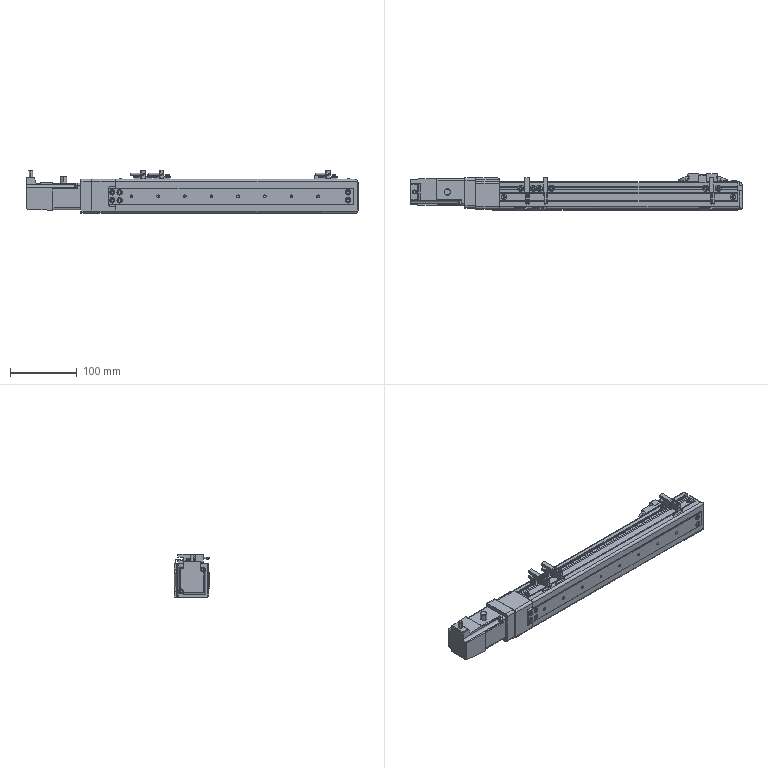Part | SolidWorks | features BaseBody 7, MoveFace 1 | 7 solids | 1135 faces | box 498.4 x 54 x 65.46 mm | volume 1022785 mm3 | plane 750 | cylinder 309 | spline 40 | cone 36 | commonest cylinder face diameters 8 x28 7 x26 2 x22 5.5 x20 3 x18 3.2 x18